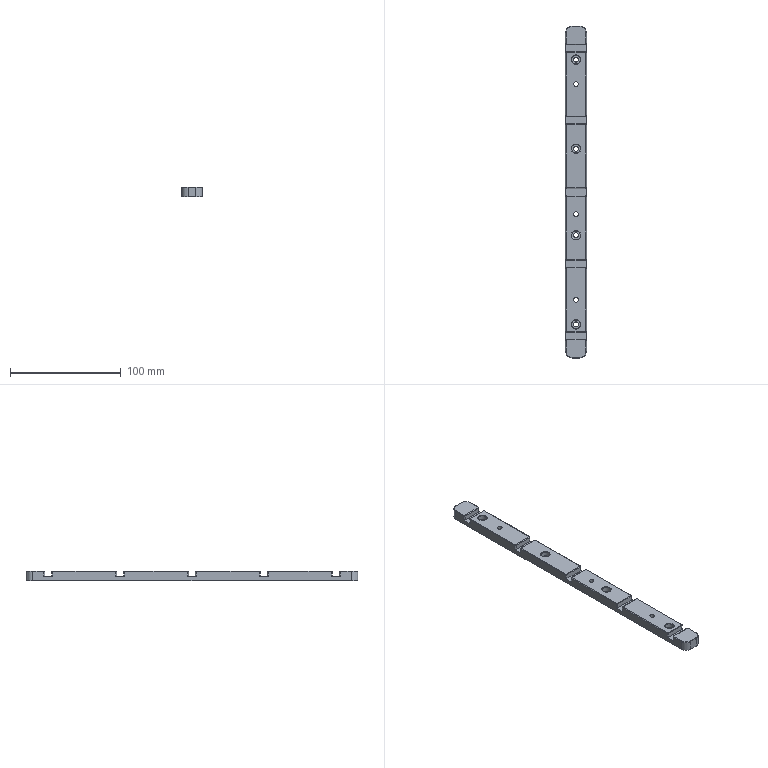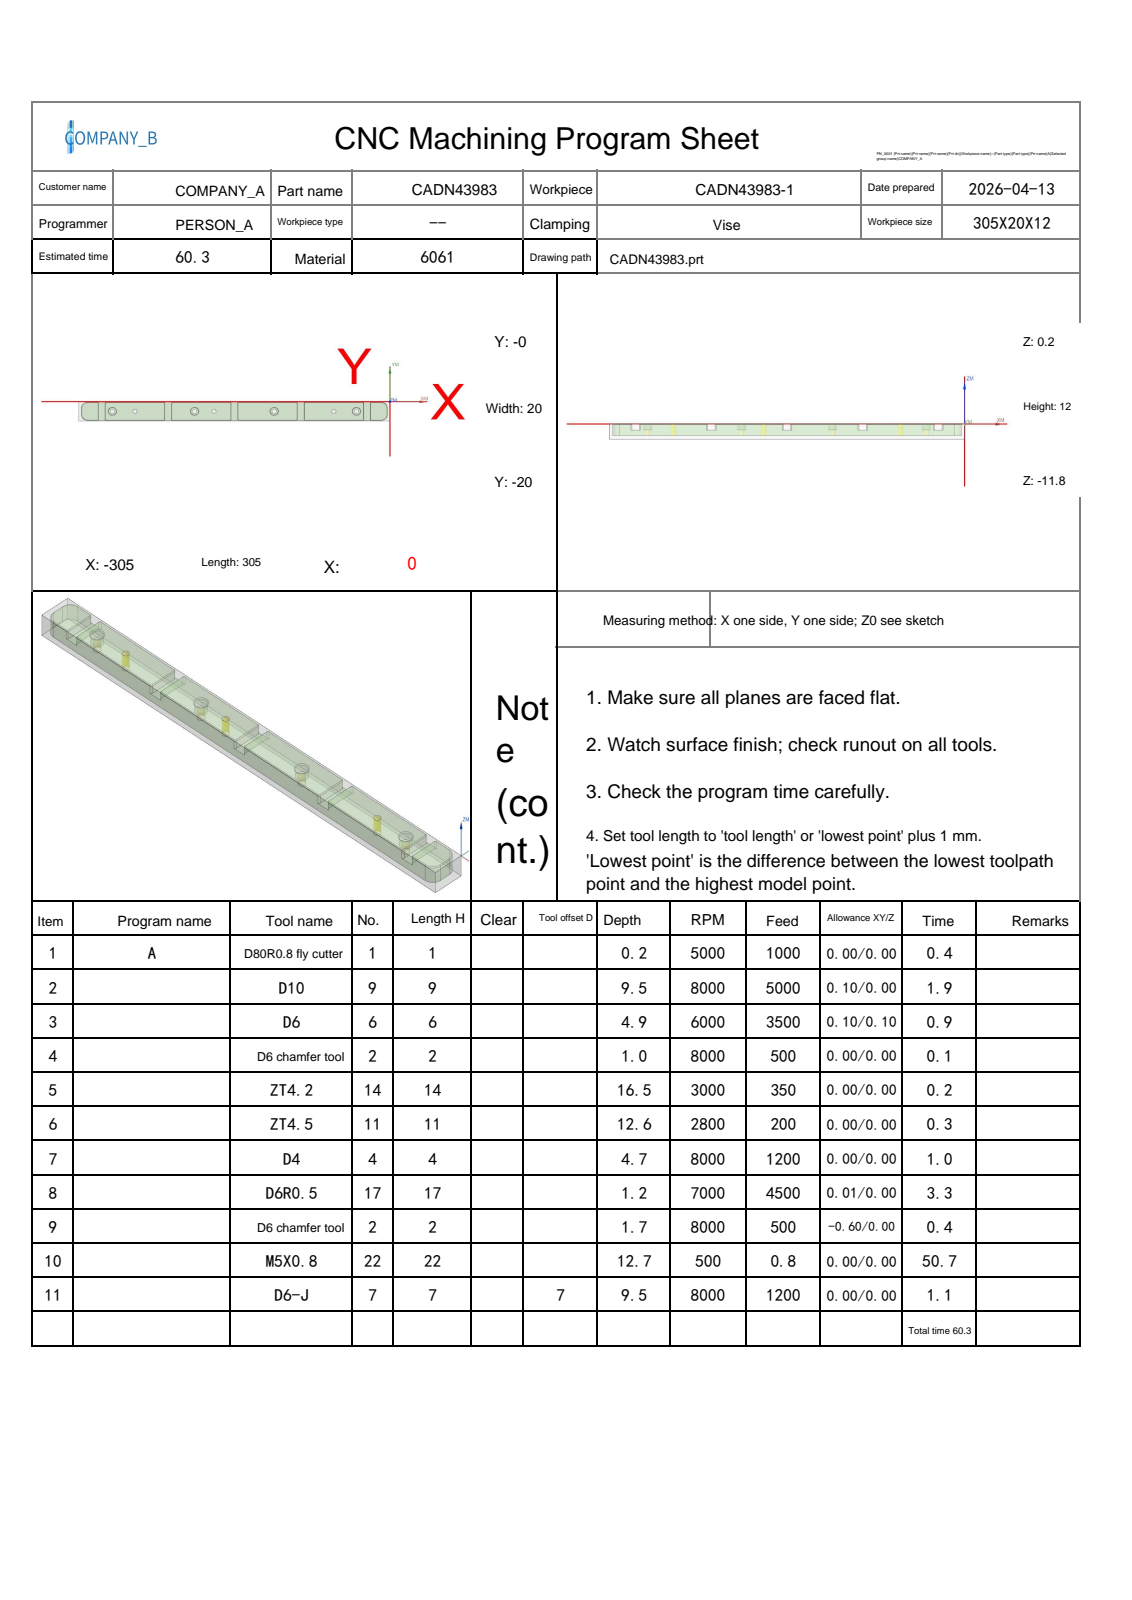NC program | NX | posted by the shop | part box 19 x 300 x 9 mm
Lines 19775 to 20188 of 20188:
N9 T02 M06
(D6 chamfer tool  D=6. R=0. H=02 ce=-0.60 di=0.00)
G00 G90 G54 X-249.306 Y-9.907 M03 S8000
G43 H02 Z20.
M08
Z-.5
G01 Z-1. F500.
X-248.5 Y-9.8
G03 X-250. Y-8.3 I-1.5 J0.0
X-251.7 Y-10. I0.0 J-1.7
X-250. Y-11.7 I1.7 J0.0
X-248.3 Y-10. I0.0 J1.7
X-250. Y-8.3 I-1.7 J0.0
X-251.5 Y-9.8 I0.0 J-1.5
G01 X-250.694 Y-9.907
Z-.5
G00 Z20.
X-171.806
Z-.5
G01 Z-1.
X-171. Y-9.8
G03 X-172.5 Y-8.3 I-1.5 J0.0
X-174.2 Y-10. I0.0 J-1.7
X-172.5 Y-11.7 I1.7 J0.0
X-170.8 Y-10. I0.0 J1.7
X-172.5 Y-8.3 I-1.7 J0.0
X-174. Y-9.8 I0.0 J-1.5
G01 X-173.194 Y-9.907
Z-.5
G00 Z20.
X-55.694 Y-10.093
Z-.5
G01 Z-1.
X-56.5 Y-10.2
G03 X-55. Y-11.7 I1.5 J0.0
X-53.3 Y-10. I0.0 J1.7
X-55. Y-8.3 I-1.7 J0.0
X-56.7 Y-10. I0.0 J-1.7
X-55. Y-11.7 I1.7 J0.0
X-53.5 Y-10.2 I0.0 J1.5
G01 X-54.306 Y-10.093
Z-.5
G00 Z20.
G00 G90 X-270.029 Y-8.191 M03 S8000
Z20.
Z2.5
G01 X-270.223 Y-7.986 Z2.397 F500.
X-270.489 Y-7.768 Z2.272
X-270.78 Y-7.584 Z2.147
X-271.091 Y-7.439 Z2.022
X-271.419 Y-7.333 Z1.896
X-271.757 Y-7.269 Z1.771
X-272.1 Y-7.247 Z1.646
X-272.443 Y-7.269 Z1.521
X-272.781 Y-7.333 Z1.395
X-273.109 Y-7.439 Z1.27
X-273.42 Y-7.584 Z1.145
X-273.711 Y-7.768 Z1.02
X-273.977 Y-7.986 Z.894
X-274.214 Y-8.236 Z.769
X-274.417 Y-8.514 Z.644
X-274.546 Y-8.736 Z.55
X-274.684 Y-9.051 Z.425
X-274.783 Y-9.381 Z.3
X-274.839 Y-9.72 Z.175
X-274.852 Y-10.064 Z.05
X-274.823 Y-10.407 Z-.076
X-274.751 Y-10.744 Z-.201
X-274.637 Y-11.068 Z-.326
X-274.484 Y-11.377 Z-.451
X-274.294 Y-11.663 Z-.577
X-274.069 Y-11.924 Z-.702
X-273.814 Y-12.154 Z-.827
X-273.532 Y-12.351 Z-.952
X-273.227 Y-12.512 Z-1.078
X-272.905 Y-12.633 Z-1.203
X-272.571 Y-12.712 Z-1.328
X-272.228 Y-12.75 Z-1.453
X-272.1 Z-1.5
G03 X-269.35 Y-10. I0.0 J2.75
X-272.1 Y-7.25 I-2.75 J0.0
X-274.85 Y-10. I0.0 J-2.75
X-272.1 Y-12.75 I2.75 J0.0
X-271.603 Y-12.705 I0.0 J2.75
G01 Z1.
G00 Z20.
X-189.429 Y-8.191
Z2.5
G01 X-189.623 Y-7.986 Z2.397
X-189.889 Y-7.768 Z2.272
X-190.18 Y-7.584 Z2.147
X-190.491 Y-7.439 Z2.022
X-190.819 Y-7.333 Z1.896
X-191.157 Y-7.269 Z1.771
X-191.5 Y-7.247 Z1.646
X-191.843 Y-7.269 Z1.521
X-192.181 Y-7.333 Z1.395
X-192.509 Y-7.439 Z1.27
X-192.82 Y-7.584 Z1.145
X-193.111 Y-7.768 Z1.02
X-193.377 Y-7.986 Z.894
X-193.614 Y-8.236 Z.769
X-193.817 Y-8.514 Z.644
X-193.946 Y-8.736 Z.55
X-194.084 Y-9.051 Z.425
X-194.183 Y-9.381 Z.3
X-194.239 Y-9.72 Z.175
X-194.252 Y-10.064 Z.05
X-194.223 Y-10.407 Z-.076
X-194.151 Y-10.744 Z-.201
X-194.037 Y-11.068 Z-.326
X-193.884 Y-11.377 Z-.451
X-193.694 Y-11.663 Z-.577
X-193.469 Y-11.924 Z-.702
X-193.214 Y-12.154 Z-.827
X-192.932 Y-12.351 Z-.952
X-192.627 Y-12.512 Z-1.078
X-192.305 Y-12.633 Z-1.203
X-191.971 Y-12.712 Z-1.328
X-191.628 Y-12.75 Z-1.453
X-191.5 Z-1.5
G03 X-188.75 Y-10. I0.0 J2.75
X-191.5 Y-7.25 I-2.75 J0.0
X-194.25 Y-10. I0.0 J-2.75
X-191.5 Y-12.75 I2.75 J0.0
X-191.003 Y-12.705 I0.0 J2.75
G01 Z1.
G00 Z20.
X-111.429 Y-8.191
Z2.5
G01 X-111.623 Y-7.986 Z2.397
X-111.889 Y-7.768 Z2.272
X-112.18 Y-7.584 Z2.147
X-112.491 Y-7.439 Z2.022
X-112.819 Y-7.333 Z1.896
X-113.157 Y-7.269 Z1.771
X-113.5 Y-7.247 Z1.646
X-113.843 Y-7.269 Z1.521
X-114.181 Y-7.333 Z1.395
X-114.509 Y-7.439 Z1.27
X-114.82 Y-7.584 Z1.145
X-115.111 Y-7.768 Z1.02
X-115.377 Y-7.986 Z.894
X-115.614 Y-8.236 Z.769
X-115.817 Y-8.514 Z.644
X-115.946 Y-8.736 Z.55
X-116.084 Y-9.051 Z.425
X-116.183 Y-9.381 Z.3
X-116.239 Y-9.72 Z.175
X-116.252 Y-10.064 Z.05
X-116.223 Y-10.407 Z-.076
X-116.151 Y-10.744 Z-.201
X-116.037 Y-11.068 Z-.326
X-115.884 Y-11.377 Z-.451
X-115.694 Y-11.663 Z-.577
X-115.469 Y-11.924 Z-.702
X-115.214 Y-12.154 Z-.827
X-114.932 Y-12.351 Z-.952
X-114.627 Y-12.512 Z-1.078
X-114.305 Y-12.633 Z-1.203
X-113.971 Y-12.712 Z-1.328
X-113.628 Y-12.75 Z-1.453
X-113.5 Z-1.5
G03 X-110.75 Y-10. I0.0 J2.75
X-113.5 Y-7.25 I-2.75 J0.0
X-116.25 Y-10. I0.0 J-2.75
X-113.5 Y-12.75 I2.75 J0.0
X-113.003 Y-12.705 I0.0 J2.75
G01 Z1.
G00 Z20.
X-30.829 Y-8.191
Z2.5
G01 X-31.023 Y-7.986 Z2.397
X-31.289 Y-7.768 Z2.272
X-31.58 Y-7.584 Z2.147
X-31.891 Y-7.439 Z2.022
X-32.219 Y-7.333 Z1.896
X-32.557 Y-7.269 Z1.771
X-32.9 Y-7.247 Z1.646
X-33.243 Y-7.269 Z1.521
X-33.581 Y-7.333 Z1.395
X-33.909 Y-7.439 Z1.27
X-34.22 Y-7.584 Z1.145
X-34.511 Y-7.768 Z1.02
X-34.777 Y-7.986 Z.894
X-35.014 Y-8.236 Z.769
X-35.217 Y-8.514 Z.644
X-35.346 Y-8.736 Z.55
X-35.484 Y-9.051 Z.425
X-35.583 Y-9.381 Z.3
X-35.639 Y-9.72 Z.175
X-35.652 Y-10.064 Z.05
X-35.623 Y-10.407 Z-.076
X-35.551 Y-10.744 Z-.201
X-35.437 Y-11.068 Z-.326
X-35.284 Y-11.377 Z-.451
X-35.094 Y-11.663 Z-.577
X-34.869 Y-11.924 Z-.702
X-34.614 Y-12.154 Z-.827
X-34.332 Y-12.351 Z-.952
X-34.027 Y-12.512 Z-1.078
X-33.705 Y-12.633 Z-1.203
X-33.371 Y-12.712 Z-1.328
X-33.028 Y-12.75 Z-1.453
X-32.9 Z-1.5
G03 X-30.15 Y-10. I0.0 J2.75
X-32.9 Y-7.25 I-2.75 J0.0
X-35.65 Y-10. I0.0 J-2.75
X-32.9 Y-12.75 I2.75 J0.0
X-32.403 Y-12.705 I0.0 J2.75
G01 Z1.
G00 Z20.
G91 G28 Z0.0
M05
M09
G91 G28 Z0.0
M01
N10 T22 M06
(M5X0.8 D=4.2 DR_a=180 H=22)
G00 G90 G54 X-55. Y-10. M03 S500
G43 H22 Z20.
M08
G95
G98 G84 X-55. Y-10. Z-12.5 R1. F.8 Q3.
X-172.5
X-250.
G80
G94
G00 Z20.
G91 G28 Z0.0
M05
M09
G91 G28 Z0.0
M01
N11 T07 M06
(D6-J  D=6. R=0. H=07 ce=0.00 di=0.00)
G00 G90 G54 X-14.65 Y-23.6 M03 S6000
G43 H07 Z20.
M08
Z-4.3
G01 Z-4.8 F1200.
G41 D07
Y-23.5
G03 X-15.65 Y-22.5 I-1. J0.0
G01 X-18.35
G02 X-22.35 Y-18.5 I0.0 J4.
G01 Y-1.5
G02 X-18.35 Y2.5 I4. J0.0
G01 X-15.65
G03 X-14.65 Y3.5 I0.0 J1.
G01 G40 Y3.6
Z-4.3
G00 Z20.
X-30.35
Z-4.3
G01 Z-4.8
G41 D07
Y3.5
G03 X-29.35 Y2.5 I1. J0.0
G01 X-26.65
G02 X-22.65 Y-1.5 I0.0 J-4.
G01 Y-18.5
G02 X-26.65 Y-22.5 I-4. J0.0
G01 X-29.35
G03 X-30.35 Y-23.5 I0.0 J-1.
G01 G40 Y-23.6
Z-4.3
G00 Z20.
X-79.65
Z-4.3
G01 Z-4.8
G41 D07
Y-23.5
G03 X-80.65 Y-22.5 I-1. J0.0
G01 X-83.35
G02 X-87.35 Y-18.5 I0.0 J4.
G01 Y-1.5
G02 X-83.35 Y2.5 I4. J0.0
G01 X-80.65
G03 X-79.65 Y3.5 I0.0 J1.
G01 G40 Y3.6
Z-4.3
G00 Z20.
X-95.35
Z-4.3
G01 Z-4.8
G41 D07
Y3.5
G03 X-94.35 Y2.5 I1. J0.0
G01 X-91.65
G02 X-87.65 Y-1.5 I0.0 J-4.
G01 Y-18.5
G02 X-91.65 Y-22.5 I-4. J0.0
G01 X-94.35
G03 X-95.35 Y-23.5 I0.0 J-1.
G01 G40 Y-23.6
Z-4.3
G00 Z20.
X-144.65
Z-4.3
G01 Z-4.8
G41 D07
Y-23.5
G03 X-145.65 Y-22.5 I-1. J0.0
G01 X-148.35
G02 X-152.35 Y-18.5 I0.0 J4.
G01 Y-1.5
G02 X-148.35 Y2.5 I4. J0.0
G01 X-145.65
G03 X-144.65 Y3.5 I0.0 J1.
G01 G40 Y3.6
Z-4.3
G00 Z20.
X-160.35
Z-4.3
G01 Z-4.8
G41 D07
Y3.5
G03 X-159.35 Y2.5 I1. J0.0
G01 X-156.65
G02 X-152.65 Y-1.5 I0.0 J-4.
G01 Y-18.5
G02 X-156.65 Y-22.5 I-4. J0.0
G01 X-159.35
G03 X-160.35 Y-23.5 I0.0 J-1.
G01 G40 Y-23.6
Z-4.3
G00 Z20.
X-209.65
Z-4.3
G01 Z-4.8
G41 D07
Y-23.5
G03 X-210.65 Y-22.5 I-1. J0.0
G01 X-213.35
G02 X-217.35 Y-18.5 I0.0 J4.
G01 Y-1.5
G02 X-213.35 Y2.5 I4. J0.0
G01 X-210.65
G03 X-209.65 Y3.5 I0.0 J1.
G01 G40 Y3.6
Z-4.3
G00 Z20.
X-225.35
Z-4.3
G01 Z-4.8
G41 D07
Y3.5
G03 X-224.35 Y2.5 I1. J0.0
G01 X-221.65
G02 X-217.65 Y-1.5 I0.0 J-4.
G01 Y-18.5
G02 X-221.65 Y-22.5 I-4. J0.0
G01 X-224.35
G03 X-225.35 Y-23.5 I0.0 J-1.
G01 G40 Y-23.6
Z-4.3
G00 Z20.
X-274.65
Z-4.3
G01 Z-4.8
G41 D07
Y-23.5
G03 X-275.65 Y-22.5 I-1. J0.0
G01 X-278.35
G02 X-282.35 Y-18.5 I0.0 J4.
G01 Y-1.5
G02 X-278.35 Y2.5 I4. J0.0
G01 X-275.65
G03 X-274.65 Y3.5 I0.0 J1.
G01 G40 Y3.6
Z-4.3
G00 Z20.
X-290.35
Z-4.3
G01 Z-4.8
G41 D07
Y3.5
G03 X-289.35 Y2.5 I1. J0.0
G01 X-286.65
G02 X-282.65 Y-1.5 I0.0 J-4.
G01 Y-18.5
G02 X-286.65 Y-22.5 I-4. J0.0
G01 X-289.35
G03 X-290.35 Y-23.5 I0.0 J-1.
G01 G40 Y-23.6
Z-4.3
G00 Z20.
G00 G90 X-297.509 Y3.65 M03 S8000
Z20.
Z-8.8
G01 Z-9.3 F1000.
G41 D07
X-297.499 Y3.45
G03 X-296.5 Y2.5 I.999 J.05
G01 X-8.5
G02 X.5 Y-6.5 I0.0 J-9.
G01 Y-13.5
G02 X-8.5 Y-22.5 I-9. J0.0
G01 X-296.5
G02 X-305.5 Y-13.5 I0.0 J9.
G01 Y-6.5
G02 X-296.5 Y2.5 I9. J0.0
G01 X-296.
G03 X-295. Y3.5 I0.0 J1.
G01 G40 Y3.7
Z-8.8
G00 Z20.
M05
M09
G91 G28 Z0.0
G91 G28 Y0.0
M30
%